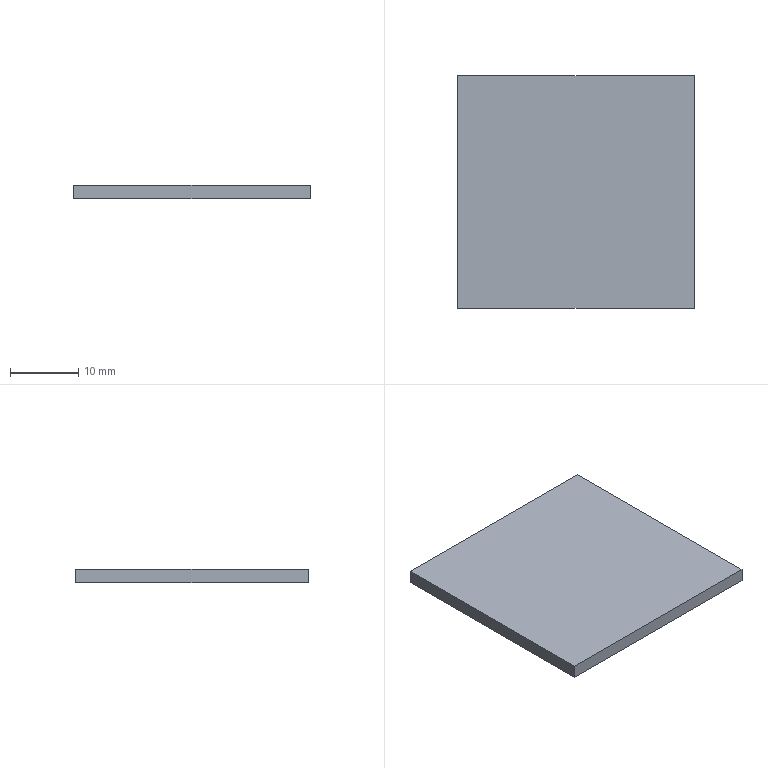Part | STEP file | ASND-0110-OPT-CO40-X-V1.0 diffuser plate | 1 solid | 6 faces | box 34.8 x 34.2 x 2 mm | volume 2380 mm3 | plane 6
STEP:
#1=CARTESIAN_POINT('',(0.,0.,0.));
#2=DIRECTION('',(0.,0.,1.));
#3=DIRECTION('',(1.,0.,0.));
#4=AXIS2_PLACEMENT_3D('',#1,#2,#3);
#5=CARTESIAN_POINT('',(-17.4,-17.1,-2.));
#6=VERTEX_POINT('',#5);
#7=CARTESIAN_POINT('',(-17.4,17.1,-2.));
#8=VERTEX_POINT('',#7);
#9=CARTESIAN_POINT('',(-17.4,-17.1,-2.));
#10=DIRECTION('',(0.,1.,0.));
#11=VECTOR('',#10,1.);
#12=LINE('',#9,#11);
#13=CARTESIAN_POINT('',(-17.4,-17.1,-2.));
#14=DIRECTION('',(-1.,0.,0.));
#15=DIRECTION('',(0.,0.7071,0.7071));
#16=AXIS2_PLACEMENT_3D('',#13,#14,#15);
#17=PLANE('',#16);
#18=CARTESIAN_POINT('',(0.,0.));
#19=DIRECTION('',(0.7071,0.7071));
#20=VECTOR('',#19,1.);
#21=LINE('',#18,#20);
#22=(GEOMETRIC_REPRESENTATION_CONTEXT(2)PARAMETRIC_REPRESENTATION_CONTEXT()REPRESENTATION_CONTEXT('',''));
#23=DEFINITIONAL_REPRESENTATION('',(#21),#22);
#24=PCURVE('',#17,#23);
#25=CARTESIAN_POINT('',(17.4,-17.1,-2.));
#26=DIRECTION('',(0.,0.,-1.));
#27=DIRECTION('',(0.7071,0.7071,0.));
#28=AXIS2_PLACEMENT_3D('',#25,#26,#27);
#29=PLANE('',#28);
#30=CARTESIAN_POINT('',(-24.607,-24.607));
#31=DIRECTION('',(0.7071,-0.7071));
#32=VECTOR('',#31,1.);
#33=LINE('',#30,#32);
#34=(GEOMETRIC_REPRESENTATION_CONTEXT(2)PARAMETRIC_REPRESENTATION_CONTEXT()REPRESENTATION_CONTEXT('',''));
#35=DEFINITIONAL_REPRESENTATION('',(#33),#34);
#36=PCURVE('',#29,#35);
#37=SURFACE_CURVE('',#12,(#24,#36),.PCURVE_S1.);
#38=EDGE_CURVE('',#6,#8,#37,.T.);
#39=ORIENTED_EDGE('',*,*,#38,.F.);
#40=CARTESIAN_POINT('',(-17.4,-17.1,0.));
#41=VERTEX_POINT('',#40);
#42=CARTESIAN_POINT('',(-17.4,-17.1,0.));
#43=DIRECTION('',(0.,0.,-1.));
#44=VECTOR('',#43,1.);
#45=LINE('',#42,#44);
#46=CARTESIAN_POINT('',(1.414,-1.414));
#47=DIRECTION('',(-0.7071,0.7071));
#48=VECTOR('',#47,1.);
#49=LINE('',#46,#48);
#50=(GEOMETRIC_REPRESENTATION_CONTEXT(2)PARAMETRIC_REPRESENTATION_CONTEXT()REPRESENTATION_CONTEXT('',''));
#51=DEFINITIONAL_REPRESENTATION('',(#49),#50);
#52=PCURVE('',#17,#51);
#53=CARTESIAN_POINT('',(-17.4,-17.1,0.));
#54=DIRECTION('',(0.,-1.,0.));
#55=DIRECTION('',(0.7071,0.,0.7071));
#56=AXIS2_PLACEMENT_3D('',#53,#54,#55);
#57=PLANE('',#56);
#58=CARTESIAN_POINT('',(0.,0.));
#59=DIRECTION('',(-0.7071,-0.7071));
#60=VECTOR('',#59,1.);
#61=LINE('',#58,#60);
#62=(GEOMETRIC_REPRESENTATION_CONTEXT(2)PARAMETRIC_REPRESENTATION_CONTEXT()REPRESENTATION_CONTEXT('',''));
#63=DEFINITIONAL_REPRESENTATION('',(#61),#62);
#64=PCURVE('',#57,#63);
#65=SURFACE_CURVE('',#45,(#52,#64),.PCURVE_S1.);
#66=EDGE_CURVE('',#41,#6,#65,.T.);
#67=ORIENTED_EDGE('',*,*,#66,.F.);
#68=CARTESIAN_POINT('',(-17.4,17.1,0.));
#69=VERTEX_POINT('',#68);
#70=CARTESIAN_POINT('',(-17.4,-17.1,0.));
#71=DIRECTION('',(0.,1.,0.));
#72=VECTOR('',#71,1.);
#73=LINE('',#70,#72);
#74=CARTESIAN_POINT('',(1.414,-1.414));
#75=DIRECTION('',(0.7071,0.7071));
#76=VECTOR('',#75,1.);
#77=LINE('',#74,#76);
#78=(GEOMETRIC_REPRESENTATION_CONTEXT(2)PARAMETRIC_REPRESENTATION_CONTEXT()REPRESENTATION_CONTEXT('',''));
#79=DEFINITIONAL_REPRESENTATION('',(#77),#78);
#80=PCURVE('',#17,#79);
#81=CARTESIAN_POINT('',(17.4,-17.1,0.));
#82=DIRECTION('',(0.,0.,-1.));
#83=DIRECTION('',(0.7071,0.7071,0.));
#84=AXIS2_PLACEMENT_3D('',#81,#82,#83);
#85=PLANE('',#84);
#86=CARTESIAN_POINT('',(-24.607,-24.607));
#87=DIRECTION('',(0.7071,-0.7071));
#88=VECTOR('',#87,1.);
#89=LINE('',#86,#88);
#90=(GEOMETRIC_REPRESENTATION_CONTEXT(2)PARAMETRIC_REPRESENTATION_CONTEXT()REPRESENTATION_CONTEXT('',''));
#91=DEFINITIONAL_REPRESENTATION('',(#89),#90);
#92=PCURVE('',#85,#91);
#93=SURFACE_CURVE('',#73,(#80,#92),.PCURVE_S1.);
#94=EDGE_CURVE('',#41,#69,#93,.T.);
#95=ORIENTED_EDGE('',*,*,#94,.T.);
#96=CARTESIAN_POINT('',(-17.4,17.1,-2.));
#97=DIRECTION('',(0.,0.,1.));
#98=VECTOR('',#97,1.);
#99=LINE('',#96,#98);
#100=CARTESIAN_POINT('',(24.183,24.183));
#101=DIRECTION('',(0.7071,-0.7071));
#102=VECTOR('',#101,1.);
#103=LINE('',#100,#102);
#104=(GEOMETRIC_REPRESENTATION_CONTEXT(2)PARAMETRIC_REPRESENTATION_CONTEXT()REPRESENTATION_CONTEXT('',''));
#105=DEFINITIONAL_REPRESENTATION('',(#103),#104);
#106=PCURVE('',#17,#105);
#107=CARTESIAN_POINT('',(-17.4,17.1,-2.));
#108=DIRECTION('',(0.,1.,0.));
#109=DIRECTION('',(0.7071,0.,0.7071));
#110=AXIS2_PLACEMENT_3D('',#107,#108,#109);
#111=PLANE('',#110);
#112=CARTESIAN_POINT('',(0.,0.));
#113=DIRECTION('',(0.7071,-0.7071));
#114=VECTOR('',#113,1.);
#115=LINE('',#112,#114);
#116=(GEOMETRIC_REPRESENTATION_CONTEXT(2)PARAMETRIC_REPRESENTATION_CONTEXT()REPRESENTATION_CONTEXT('',''));
#117=DEFINITIONAL_REPRESENTATION('',(#115),#116);
#118=PCURVE('',#111,#117);
#119=SURFACE_CURVE('',#99,(#106,#118),.PCURVE_S1.);
#120=EDGE_CURVE('',#8,#69,#119,.T.);
#121=ORIENTED_EDGE('',*,*,#120,.F.);
#122=EDGE_LOOP('',(#39,#67,#95,#121));
#123=FACE_BOUND('',#122,.T.);
#124=ADVANCED_FACE('',(#123),#17,.T.);
#125=CARTESIAN_POINT('',(17.4,17.1,0.));
#126=VERTEX_POINT('',#125);
#127=CARTESIAN_POINT('',(-17.4,17.1,0.));
#128=DIRECTION('',(1.,0.,0.));
#129=VECTOR('',#128,1.);
#130=LINE('',#127,#129);
#131=CARTESIAN_POINT('',(-0.4243,-48.79));
#132=DIRECTION('',(0.7071,0.7071));
#133=VECTOR('',#132,1.);
#134=LINE('',#131,#133);
#135=(GEOMETRIC_REPRESENTATION_CONTEXT(2)PARAMETRIC_REPRESENTATION_CONTEXT()REPRESENTATION_CONTEXT('',''));
#136=DEFINITIONAL_REPRESENTATION('',(#134),#135);
#137=PCURVE('',#85,#136);
#138=CARTESIAN_POINT('',(1.414,-1.414));
#139=DIRECTION('',(0.7071,0.7071));
#140=VECTOR('',#139,1.);
#141=LINE('',#138,#140);
#142=(GEOMETRIC_REPRESENTATION_CONTEXT(2)PARAMETRIC_REPRESENTATION_CONTEXT()REPRESENTATION_CONTEXT('',''));
#143=DEFINITIONAL_REPRESENTATION('',(#141),#142);
#144=PCURVE('',#111,#143);
#145=SURFACE_CURVE('',#130,(#137,#144),.PCURVE_S1.);
#146=EDGE_CURVE('',#69,#126,#145,.T.);
#147=ORIENTED_EDGE('',*,*,#146,.F.);
#148=ORIENTED_EDGE('',*,*,#94,.F.);
#149=CARTESIAN_POINT('',(17.4,-17.1,0.));
#150=VERTEX_POINT('',#149);
#151=CARTESIAN_POINT('',(17.4,-17.1,0.));
#152=DIRECTION('',(-1.,0.,0.));
#153=VECTOR('',#152,1.);
#154=LINE('',#151,#153);
#155=CARTESIAN_POINT('',(0.,0.));
#156=DIRECTION('',(-0.7071,-0.7071));
#157=VECTOR('',#156,1.);
#158=LINE('',#155,#157);
#159=(GEOMETRIC_REPRESENTATION_CONTEXT(2)PARAMETRIC_REPRESENTATION_CONTEXT()REPRESENTATION_CONTEXT('',''));
#160=DEFINITIONAL_REPRESENTATION('',(#158),#159);
#161=PCURVE('',#85,#160);
#162=CARTESIAN_POINT('',(24.607,-24.607));
#163=DIRECTION('',(-0.7071,0.7071));
#164=VECTOR('',#163,1.);
#165=LINE('',#162,#164);
#166=(GEOMETRIC_REPRESENTATION_CONTEXT(2)PARAMETRIC_REPRESENTATION_CONTEXT()REPRESENTATION_CONTEXT('',''));
#167=DEFINITIONAL_REPRESENTATION('',(#165),#166);
#168=PCURVE('',#57,#167);
#169=SURFACE_CURVE('',#154,(#161,#168),.PCURVE_S1.);
#170=EDGE_CURVE('',#150,#41,#169,.T.);
#171=ORIENTED_EDGE('',*,*,#170,.F.);
#172=CARTESIAN_POINT('',(17.4,17.1,0.));
#173=DIRECTION('',(0.,-1.,0.));
#174=VECTOR('',#173,1.);
#175=LINE('',#172,#174);
#176=CARTESIAN_POINT('',(24.183,-24.183));
#177=DIRECTION('',(-0.7071,0.7071));
#178=VECTOR('',#177,1.);
#179=LINE('',#176,#178);
#180=(GEOMETRIC_REPRESENTATION_CONTEXT(2)PARAMETRIC_REPRESENTATION_CONTEXT()REPRESENTATION_CONTEXT('',''));
#181=DEFINITIONAL_REPRESENTATION('',(#179),#180);
#182=PCURVE('',#85,#181);
#183=CARTESIAN_POINT('',(17.4,-17.1,0.));
#184=DIRECTION('',(1.,0.,0.));
#185=DIRECTION('',(0.,0.7071,0.7071));
#186=AXIS2_PLACEMENT_3D('',#183,#184,#185);
#187=PLANE('',#186);
#188=CARTESIAN_POINT('',(24.183,-24.183));
#189=DIRECTION('',(-0.7071,0.7071));
#190=VECTOR('',#189,1.);
#191=LINE('',#188,#190);
#192=(GEOMETRIC_REPRESENTATION_CONTEXT(2)PARAMETRIC_REPRESENTATION_CONTEXT()REPRESENTATION_CONTEXT('',''));
#193=DEFINITIONAL_REPRESENTATION('',(#191),#192);
#194=PCURVE('',#187,#193);
#195=SURFACE_CURVE('',#175,(#182,#194),.PCURVE_S1.);
#196=EDGE_CURVE('',#126,#150,#195,.T.);
#197=ORIENTED_EDGE('',*,*,#196,.F.);
#198=EDGE_LOOP('',(#147,#148,#171,#197));
#199=FACE_BOUND('',#198,.T.);
#200=ADVANCED_FACE('',(#199),#85,.F.);
#201=CARTESIAN_POINT('',(17.4,-17.1,-2.));
#202=VERTEX_POINT('',#201);
#203=CARTESIAN_POINT('',(17.4,-17.1,-2.));
#204=DIRECTION('',(-1.,0.,0.));
#205=VECTOR('',#204,1.);
#206=LINE('',#203,#205);
#207=CARTESIAN_POINT('',(23.193,-26.022));
#208=DIRECTION('',(-0.7071,0.7071));
#209=VECTOR('',#208,1.);
#210=LINE('',#207,#209);
#211=(GEOMETRIC_REPRESENTATION_CONTEXT(2)PARAMETRIC_REPRESENTATION_CONTEXT()REPRESENTATION_CONTEXT('',''));
#212=DEFINITIONAL_REPRESENTATION('',(#210),#211);
#213=PCURVE('',#57,#212);
#214=CARTESIAN_POINT('',(0.,0.));
#215=DIRECTION('',(-0.7071,-0.7071));
#216=VECTOR('',#215,1.);
#217=LINE('',#214,#216);
#218=(GEOMETRIC_REPRESENTATION_CONTEXT(2)PARAMETRIC_REPRESENTATION_CONTEXT()REPRESENTATION_CONTEXT('',''));
#219=DEFINITIONAL_REPRESENTATION('',(#217),#218);
#220=PCURVE('',#29,#219);
#221=SURFACE_CURVE('',#206,(#213,#220),.PCURVE_S1.);
#222=EDGE_CURVE('',#202,#6,#221,.T.);
#223=ORIENTED_EDGE('',*,*,#222,.F.);
#224=CARTESIAN_POINT('',(17.4,-17.1,0.));
#225=DIRECTION('',(0.,0.,-1.));
#226=VECTOR('',#225,1.);
#227=LINE('',#224,#226);
#228=CARTESIAN_POINT('',(24.607,-24.607));
#229=DIRECTION('',(-0.7071,-0.7071));
#230=VECTOR('',#229,1.);
#231=LINE('',#228,#230);
#232=(GEOMETRIC_REPRESENTATION_CONTEXT(2)PARAMETRIC_REPRESENTATION_CONTEXT()REPRESENTATION_CONTEXT('',''));
#233=DEFINITIONAL_REPRESENTATION('',(#231),#232);
#234=PCURVE('',#57,#233);
#235=CARTESIAN_POINT('',(0.,0.));
#236=DIRECTION('',(-0.7071,-0.7071));
#237=VECTOR('',#236,1.);
#238=LINE('',#235,#237);
#239=(GEOMETRIC_REPRESENTATION_CONTEXT(2)PARAMETRIC_REPRESENTATION_CONTEXT()REPRESENTATION_CONTEXT('',''));
#240=DEFINITIONAL_REPRESENTATION('',(#238),#239);
#241=PCURVE('',#187,#240);
#242=SURFACE_CURVE('',#227,(#234,#241),.PCURVE_S1.);
#243=EDGE_CURVE('',#150,#202,#242,.T.);
#244=ORIENTED_EDGE('',*,*,#243,.F.);
#245=ORIENTED_EDGE('',*,*,#170,.T.);
#246=ORIENTED_EDGE('',*,*,#66,.T.);
#247=EDGE_LOOP('',(#223,#244,#245,#246));
#248=FACE_BOUND('',#247,.T.);
#249=ADVANCED_FACE('',(#248),#57,.T.);
#250=ORIENTED_EDGE('',*,*,#38,.T.);
#251=CARTESIAN_POINT('',(17.4,17.1,-2.));
#252=VERTEX_POINT('',#251);
#253=CARTESIAN_POINT('',(17.4,17.1,-2.));
#254=DIRECTION('',(-1.,0.,0.));
#255=VECTOR('',#254,1.);
#256=LINE('',#253,#255);
#257=CARTESIAN_POINT('',(24.183,-24.183));
#258=DIRECTION('',(-0.7071,-0.7071));
#259=VECTOR('',#258,1.);
#260=LINE('',#257,#259);
#261=(GEOMETRIC_REPRESENTATION_CONTEXT(2)PARAMETRIC_REPRESENTATION_CONTEXT()REPRESENTATION_CONTEXT('',''));
#262=DEFINITIONAL_REPRESENTATION('',(#260),#261);
#263=PCURVE('',#29,#262);
#264=CARTESIAN_POINT('',(24.607,24.607));
#265=DIRECTION('',(-0.7071,-0.7071));
#266=VECTOR('',#265,1.);
#267=LINE('',#264,#266);
#268=(GEOMETRIC_REPRESENTATION_CONTEXT(2)PARAMETRIC_REPRESENTATION_CONTEXT()REPRESENTATION_CONTEXT('',''));
#269=DEFINITIONAL_REPRESENTATION('',(#267),#268);
#270=PCURVE('',#111,#269);
#271=SURFACE_CURVE('',#256,(#263,#270),.PCURVE_S1.);
#272=EDGE_CURVE('',#252,#8,#271,.T.);
#273=ORIENTED_EDGE('',*,*,#272,.F.);
#274=CARTESIAN_POINT('',(17.4,-17.1,-2.));
#275=DIRECTION('',(0.,1.,0.));
#276=VECTOR('',#275,1.);
#277=LINE('',#274,#276);
#278=CARTESIAN_POINT('',(0.,0.));
#279=DIRECTION('',(0.7071,-0.7071));
#280=VECTOR('',#279,1.);
#281=LINE('',#278,#280);
#282=(GEOMETRIC_REPRESENTATION_CONTEXT(2)PARAMETRIC_REPRESENTATION_CONTEXT()REPRESENTATION_CONTEXT('',''));
#283=DEFINITIONAL_REPRESENTATION('',(#281),#282);
#284=PCURVE('',#29,#283);
#285=CARTESIAN_POINT('',(-1.414,-1.414));
#286=DIRECTION('',(0.7071,-0.7071));
#287=VECTOR('',#286,1.);
#288=LINE('',#285,#287);
#289=(GEOMETRIC_REPRESENTATION_CONTEXT(2)PARAMETRIC_REPRESENTATION_CONTEXT()REPRESENTATION_CONTEXT('',''));
#290=DEFINITIONAL_REPRESENTATION('',(#288),#289);
#291=PCURVE('',#187,#290);
#292=SURFACE_CURVE('',#277,(#284,#291),.PCURVE_S1.);
#293=EDGE_CURVE('',#202,#252,#292,.T.);
#294=ORIENTED_EDGE('',*,*,#293,.F.);
#295=ORIENTED_EDGE('',*,*,#222,.T.);
#296=EDGE_LOOP('',(#250,#273,#294,#295));
#297=FACE_BOUND('',#296,.T.);
#298=ADVANCED_FACE('',(#297),#29,.T.);
#299=ORIENTED_EDGE('',*,*,#272,.T.);
#300=ORIENTED_EDGE('',*,*,#120,.T.);
#301=ORIENTED_EDGE('',*,*,#146,.T.);
#302=CARTESIAN_POINT('',(17.4,17.1,-2.));
#303=DIRECTION('',(0.,0.,1.));
#304=VECTOR('',#303,1.);
#305=LINE('',#302,#304);
#306=CARTESIAN_POINT('',(24.607,24.607));
#307=DIRECTION('',(0.7071,-0.7071));
#308=VECTOR('',#307,1.);
#309=LINE('',#306,#308);
#310=(GEOMETRIC_REPRESENTATION_CONTEXT(2)PARAMETRIC_REPRESENTATION_CONTEXT()REPRESENTATION_CONTEXT('',''));
#311=DEFINITIONAL_REPRESENTATION('',(#309),#310);
#312=PCURVE('',#111,#311);
#313=CARTESIAN_POINT('',(22.769,-25.597));
#314=DIRECTION('',(0.7071,0.7071));
#315=VECTOR('',#314,1.);
#316=LINE('',#313,#315);
#317=(GEOMETRIC_REPRESENTATION_CONTEXT(2)PARAMETRIC_REPRESENTATION_CONTEXT()REPRESENTATION_CONTEXT('',''));
#318=DEFINITIONAL_REPRESENTATION('',(#316),#317);
#319=PCURVE('',#187,#318);
#320=SURFACE_CURVE('',#305,(#312,#319),.PCURVE_S1.);
#321=EDGE_CURVE('',#252,#126,#320,.T.);
#322=ORIENTED_EDGE('',*,*,#321,.F.);
#323=EDGE_LOOP('',(#299,#300,#301,#322));
#324=FACE_BOUND('',#323,.T.);
#325=ADVANCED_FACE('',(#324),#111,.T.);
#326=ORIENTED_EDGE('',*,*,#293,.T.);
#327=ORIENTED_EDGE('',*,*,#321,.T.);
#328=ORIENTED_EDGE('',*,*,#196,.T.);
#329=ORIENTED_EDGE('',*,*,#243,.T.);
#330=EDGE_LOOP('',(#326,#327,#328,#329));
#331=FACE_BOUND('',#330,.T.);
#332=ADVANCED_FACE('',(#331),#187,.T.);
#333=CLOSED_SHELL('',(#124,#200,#249,#298,#325,#332));
#334=MANIFOLD_SOLID_BREP('',#333);
#335=(LENGTH_UNIT()NAMED_UNIT(*)SI_UNIT(.MILLI.,.METRE.));
#336=UNCERTAINTY_MEASURE_WITH_UNIT(LENGTH_MEASURE(0.0000001),#335,'','');
#337=(NAMED_UNIT(*)PLANE_ANGLE_UNIT()SI_UNIT($,.RADIAN.));
#338=(NAMED_UNIT(*)SI_UNIT($,.STERADIAN.)SOLID_ANGLE_UNIT());
#339=(GEOMETRIC_REPRESENTATION_CONTEXT(3)GLOBAL_UNCERTAINTY_ASSIGNED_CONTEXT((#336))GLOBAL_UNIT_ASSIGNED_CONTEXT((#335,#337,#338))REPRESENTATION_CONTEXT('',''));
#340=ADVANCED_BREP_SHAPE_REPRESENTATION('',(#4,#334),#339);